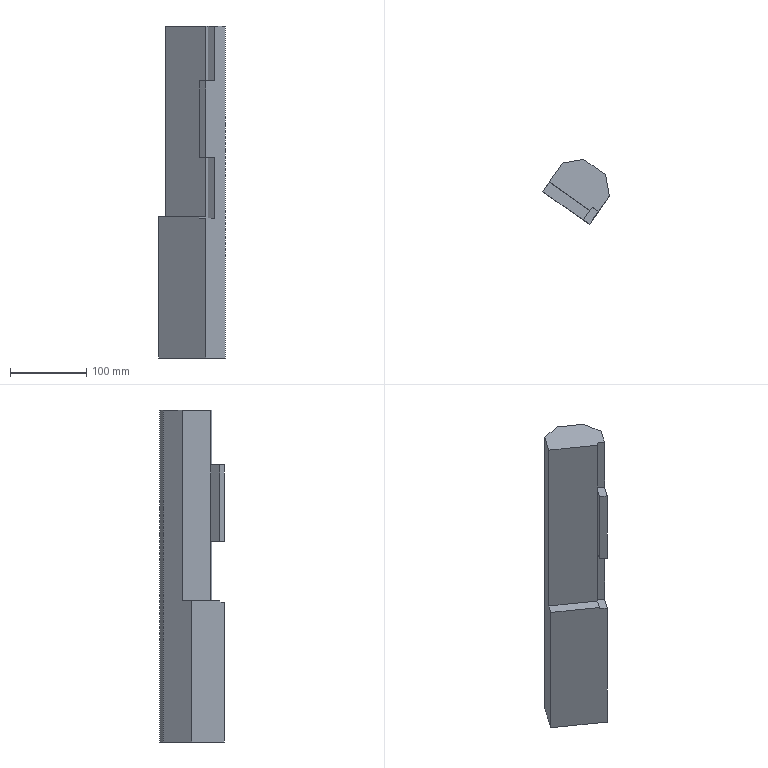Part | NX | features solid 2 | 1 solid | 19 faces | box 87.247 x 84.792 x 435 mm | volume 1672471 mm3 | plane 19
STEP:
#1=CARTESIAN_POINT('',(329.008,618.065,-154.062));
#2=VERTEX_POINT('',#1);
#3=CARTESIAN_POINT('',(357.678,597.989,-154.062));
#4=VERTEX_POINT('',#3);
#5=CARTESIAN_POINT('',(-199.131,987.872,-154.062));
#6=DIRECTION('',(0.8192,-0.5736,0.));
#7=VECTOR('',#6,1000.);
#8=LINE('',#5,#7);
#9=EDGE_CURVE('',#2,#4,#8,.T.);
#10=ORIENTED_EDGE('',*,*,#9,.F.);
#11=CARTESIAN_POINT('',(301.153,613.153,-154.062));
#12=VERTEX_POINT('',#11);
#13=CARTESIAN_POINT('',(301.153,613.153,-154.062));
#14=DIRECTION('',(-0.9848,-0.1736,0.));
#15=VECTOR('',#14,1000.);
#16=LINE('',#13,#15);
#17=EDGE_CURVE('',#2,#12,#16,.T.);
#18=ORIENTED_EDGE('',*,*,#17,.T.);
#19=CARTESIAN_POINT('',(283.946,588.579,-154.062));
#20=VERTEX_POINT('',#19);
#21=CARTESIAN_POINT('',(283.946,588.579,-154.062));
#22=DIRECTION('',(0.5736,0.8192,0.));
#23=VECTOR('',#22,1000.);
#24=LINE('',#21,#23);
#25=EDGE_CURVE('',#20,#12,#24,.T.);
#26=ORIENTED_EDGE('',*,*,#25,.F.);
#27=CARTESIAN_POINT('',(337.191,551.296,-154.062));
#28=VERTEX_POINT('',#27);
#29=CARTESIAN_POINT('',(283.946,588.579,-154.062));
#30=DIRECTION('',(0.8192,-0.5736,0.));
#31=VECTOR('',#30,1000.);
#32=LINE('',#29,#31);
#33=EDGE_CURVE('',#20,#28,#32,.T.);
#34=ORIENTED_EDGE('',*,*,#33,.T.);
#35=CARTESIAN_POINT('',(340.059,555.392,-154.062));
#36=VERTEX_POINT('',#35);
#37=CARTESIAN_POINT('',(337.191,551.296,-154.062));
#38=DIRECTION('',(-0.5736,-0.8192,0.));
#39=VECTOR('',#38,1000.);
#40=LINE('',#37,#39);
#41=EDGE_CURVE('',#36,#28,#40,.T.);
#42=ORIENTED_EDGE('',*,*,#41,.F.);
#43=CARTESIAN_POINT('',(348.25,549.656,-154.062));
#44=VERTEX_POINT('',#43);
#45=CARTESIAN_POINT('',(286.814,592.674,-154.062));
#46=DIRECTION('',(0.8192,-0.5736,0.));
#47=VECTOR('',#46,1000.);
#48=LINE('',#45,#47);
#49=EDGE_CURVE('',#36,#44,#48,.T.);
#50=ORIENTED_EDGE('',*,*,#49,.T.);
#51=CARTESIAN_POINT('',(362.59,570.135,-154.062));
#52=VERTEX_POINT('',#51);
#53=CARTESIAN_POINT('',(345.382,545.56,-154.062));
#54=DIRECTION('',(-0.5736,-0.8192,0.));
#55=VECTOR('',#54,1000.);
#56=LINE('',#53,#55);
#57=EDGE_CURVE('',#44,#52,#56,.F.);
#58=ORIENTED_EDGE('',*,*,#57,.T.);
#59=CARTESIAN_POINT('',(357.678,597.989,-154.062));
#60=DIRECTION('',(-0.1736,0.9848,0.));
#61=VECTOR('',#60,1000.);
#62=LINE('',#59,#61);
#63=EDGE_CURVE('',#52,#4,#62,.T.);
#64=ORIENTED_EDGE('',*,*,#63,.T.);
#65=EDGE_LOOP('',(#10,#18,#26,#34,#42,#50,#58,#64));
#66=FACE_BOUND('',#65,.T.);
#67=CARTESIAN_POINT('',(283.946,588.579,-154.062));
#68=DIRECTION('',(0.,0.,-1.));
#69=DIRECTION('',(0.5736,0.8192,0.));
#70=AXIS2_PLACEMENT_3D('',#67,#68,#69);
#71=PLANE('',#70);
#72=ADVANCED_FACE('',(#66),#71,.F.);
#73=CARTESIAN_POINT('',(337.191,551.296,-226.082));
#74=VERTEX_POINT('',#73);
#75=CARTESIAN_POINT('',(337.191,551.296,-326.082));
#76=VERTEX_POINT('',#75);
#77=CARTESIAN_POINT('',(337.191,551.296,-401.082));
#78=DIRECTION('',(0.,0.,-1.));
#79=VECTOR('',#78,1000.);
#80=LINE('',#77,#79);
#81=EDGE_CURVE('',#74,#76,#80,.T.);
#82=ORIENTED_EDGE('',*,*,#81,.F.);
#83=CARTESIAN_POINT('',(337.191,551.296,-401.082));
#84=DIRECTION('',(0.,0.,1.));
#85=VECTOR('',#84,1000.);
#86=LINE('',#83,#85);
#87=EDGE_CURVE('',#74,#28,#86,.T.);
#88=ORIENTED_EDGE('',*,*,#87,.T.);
#89=ORIENTED_EDGE('',*,*,#33,.F.);
#90=CARTESIAN_POINT('',(283.946,588.579,-404.062));
#91=VERTEX_POINT('',#90);
#92=CARTESIAN_POINT('',(283.946,588.579,-401.082));
#93=DIRECTION('',(0.,0.,-1.));
#94=VECTOR('',#93,1000.);
#95=LINE('',#92,#94);
#96=EDGE_CURVE('',#20,#91,#95,.T.);
#97=ORIENTED_EDGE('',*,*,#96,.T.);
#98=CARTESIAN_POINT('',(337.191,551.296,-404.062));
#99=VERTEX_POINT('',#98);
#100=CARTESIAN_POINT('',(283.946,588.579,-404.062));
#101=DIRECTION('',(-0.8192,0.5736,0.));
#102=VECTOR('',#101,1000.);
#103=LINE('',#100,#102);
#104=EDGE_CURVE('',#99,#91,#103,.T.);
#105=ORIENTED_EDGE('',*,*,#104,.F.);
#106=CARTESIAN_POINT('',(337.191,551.296,-401.082));
#107=DIRECTION('',(0.,0.,-1.));
#108=VECTOR('',#107,1000.);
#109=LINE('',#106,#108);
#110=EDGE_CURVE('',#76,#99,#109,.T.);
#111=ORIENTED_EDGE('',*,*,#110,.F.);
#112=EDGE_LOOP('',(#82,#88,#89,#97,#105,#111));
#113=FACE_BOUND('',#112,.T.);
#114=CARTESIAN_POINT('',(283.946,588.579,-401.082));
#115=DIRECTION('',(0.5736,0.8192,0.));
#116=DIRECTION('',(0.8192,-0.5736,0.));
#117=AXIS2_PLACEMENT_3D('',#114,#115,#116);
#118=PLANE('',#117);
#119=ADVANCED_FACE('',(#113),#118,.F.);
#120=CARTESIAN_POINT('',(328.587,539.009,-404.062));
#121=VERTEX_POINT('',#120);
#122=CARTESIAN_POINT('',(328.587,539.009,-406.082));
#123=VERTEX_POINT('',#122);
#124=CARTESIAN_POINT('',(328.587,539.009,-326.082));
#125=DIRECTION('',(0.,0.,-1.));
#126=VECTOR('',#125,1000.);
#127=LINE('',#124,#126);
#128=EDGE_CURVE('',#121,#123,#127,.T.);
#129=ORIENTED_EDGE('',*,*,#128,.F.);
#130=CARTESIAN_POINT('',(275.342,576.291,-404.062));
#131=VERTEX_POINT('',#130);
#132=CARTESIAN_POINT('',(328.587,539.009,-404.062));
#133=DIRECTION('',(-0.8192,0.5736,0.));
#134=VECTOR('',#133,1000.);
#135=LINE('',#132,#134);
#136=EDGE_CURVE('',#121,#131,#135,.T.);
#137=ORIENTED_EDGE('',*,*,#136,.T.);
#138=CARTESIAN_POINT('',(275.342,576.291,-589.062));
#139=VERTEX_POINT('',#138);
#140=CARTESIAN_POINT('',(275.342,576.291,-401.082));
#141=DIRECTION('',(0.,0.,-1.));
#142=VECTOR('',#141,1000.);
#143=LINE('',#140,#142);
#144=EDGE_CURVE('',#131,#139,#143,.T.);
#145=ORIENTED_EDGE('',*,*,#144,.T.);
#146=CARTESIAN_POINT('',(336.779,533.273,-589.062));
#147=VERTEX_POINT('',#146);
#148=CARTESIAN_POINT('',(275.26,576.349,-589.062));
#149=DIRECTION('',(0.8192,-0.5736,0.));
#150=VECTOR('',#149,1000.);
#151=LINE('',#148,#150);
#152=EDGE_CURVE('',#147,#139,#151,.F.);
#153=ORIENTED_EDGE('',*,*,#152,.F.);
#154=CARTESIAN_POINT('',(336.779,533.273,-406.082));
#155=VERTEX_POINT('',#154);
#156=CARTESIAN_POINT('',(336.779,533.273,-461.082));
#157=DIRECTION('',(0.,0.,1.));
#158=VECTOR('',#157,1000.);
#159=LINE('',#156,#158);
#160=EDGE_CURVE('',#155,#147,#159,.F.);
#161=ORIENTED_EDGE('',*,*,#160,.F.);
#162=CARTESIAN_POINT('',(328.587,539.009,-406.082));
#163=DIRECTION('',(0.8192,-0.5736,0.));
#164=VECTOR('',#163,1000.);
#165=LINE('',#162,#164);
#166=EDGE_CURVE('',#123,#155,#165,.T.);
#167=ORIENTED_EDGE('',*,*,#166,.F.);
#168=EDGE_LOOP('',(#129,#137,#145,#153,#161,#167));
#169=FACE_BOUND('',#168,.T.);
#170=CARTESIAN_POINT('',(328.587,539.009,-461.082));
#171=DIRECTION('',(-0.5736,-0.8192,0.));
#172=DIRECTION('',(-0.8192,0.5736,0.));
#173=AXIS2_PLACEMENT_3D('',#170,#171,#172);
#174=PLANE('',#173);
#175=ADVANCED_FACE('',(#169),#174,.T.);
#176=CARTESIAN_POINT('',(301.153,613.153,-589.062));
#177=VERTEX_POINT('',#176);
#178=CARTESIAN_POINT('',(344.171,674.59,-589.062));
#179=DIRECTION('',(-0.5736,-0.8192,0.));
#180=VECTOR('',#179,1000.);
#181=LINE('',#178,#180);
#182=EDGE_CURVE('',#139,#177,#181,.F.);
#183=ORIENTED_EDGE('',*,*,#182,.T.);
#184=CARTESIAN_POINT('',(329.008,618.065,-589.062));
#185=VERTEX_POINT('',#184);
#186=CARTESIAN_POINT('',(301.153,613.153,-589.062));
#187=DIRECTION('',(-0.9848,-0.1736,0.));
#188=VECTOR('',#187,1000.);
#189=LINE('',#186,#188);
#190=EDGE_CURVE('',#177,#185,#189,.F.);
#191=ORIENTED_EDGE('',*,*,#190,.T.);
#192=CARTESIAN_POINT('',(357.678,597.989,-589.062));
#193=VERTEX_POINT('',#192);
#194=CARTESIAN_POINT('',(-199.131,987.872,-589.062));
#195=DIRECTION('',(0.8192,-0.5736,0.));
#196=VECTOR('',#195,1000.);
#197=LINE('',#194,#196);
#198=EDGE_CURVE('',#193,#185,#197,.F.);
#199=ORIENTED_EDGE('',*,*,#198,.F.);
#200=CARTESIAN_POINT('',(362.59,570.135,-589.062));
#201=VERTEX_POINT('',#200);
#202=CARTESIAN_POINT('',(357.678,597.989,-589.062));
#203=DIRECTION('',(-0.1736,0.9848,0.));
#204=VECTOR('',#203,1000.);
#205=LINE('',#202,#204);
#206=EDGE_CURVE('',#193,#201,#205,.F.);
#207=ORIENTED_EDGE('',*,*,#206,.T.);
#208=CARTESIAN_POINT('',(256.478,418.592,-589.062));
#209=DIRECTION('',(0.5736,0.8192,0.));
#210=VECTOR('',#209,1000.);
#211=LINE('',#208,#210);
#212=EDGE_CURVE('',#147,#201,#211,.T.);
#213=ORIENTED_EDGE('',*,*,#212,.F.);
#214=ORIENTED_EDGE('',*,*,#152,.T.);
#215=EDGE_LOOP('',(#183,#191,#199,#207,#213,#214));
#216=FACE_BOUND('',#215,.T.);
#217=CARTESIAN_POINT('',(344.089,674.647,-589.062));
#218=DIRECTION('',(0.,0.,-1.));
#219=DIRECTION('',(-0.5736,-0.8192,0.));
#220=AXIS2_PLACEMENT_3D('',#217,#218,#219);
#221=PLANE('',#220);
#222=ADVANCED_FACE('',(#216),#221,.T.);
#223=ORIENTED_EDGE('',*,*,#25,.T.);
#224=CARTESIAN_POINT('',(301.153,613.153,-589.062));
#225=DIRECTION('',(0.,0.,-1.));
#226=VECTOR('',#225,1000.);
#227=LINE('',#224,#226);
#228=EDGE_CURVE('',#12,#177,#227,.T.);
#229=ORIENTED_EDGE('',*,*,#228,.T.);
#230=ORIENTED_EDGE('',*,*,#182,.F.);
#231=ORIENTED_EDGE('',*,*,#144,.F.);
#232=CARTESIAN_POINT('',(283.946,588.579,-404.062));
#233=DIRECTION('',(0.5736,0.8192,0.));
#234=VECTOR('',#233,1000.);
#235=LINE('',#232,#234);
#236=EDGE_CURVE('',#131,#91,#235,.T.);
#237=ORIENTED_EDGE('',*,*,#236,.T.);
#238=ORIENTED_EDGE('',*,*,#96,.F.);
#239=EDGE_LOOP('',(#223,#229,#230,#231,#237,#238));
#240=FACE_BOUND('',#239,.T.);
#241=CARTESIAN_POINT('',(283.946,588.579,-151.082));
#242=DIRECTION('',(-0.8192,0.5736,0.));
#243=DIRECTION('',(0.5736,0.8192,0.));
#244=AXIS2_PLACEMENT_3D('',#241,#242,#243);
#245=PLANE('',#244);
#246=ADVANCED_FACE('',(#240),#245,.T.);
#247=ORIENTED_EDGE('',*,*,#198,.T.);
#248=CARTESIAN_POINT('',(329.008,618.065,-154.062));
#249=DIRECTION('',(0.,0.,1.));
#250=VECTOR('',#249,1000.);
#251=LINE('',#248,#250);
#252=EDGE_CURVE('',#185,#2,#251,.T.);
#253=ORIENTED_EDGE('',*,*,#252,.T.);
#254=ORIENTED_EDGE('',*,*,#9,.T.);
#255=CARTESIAN_POINT('',(357.678,597.989,-192.696));
#256=DIRECTION('',(0.,0.,-1.));
#257=VECTOR('',#256,1000.);
#258=LINE('',#255,#257);
#259=EDGE_CURVE('',#4,#193,#258,.T.);
#260=ORIENTED_EDGE('',*,*,#259,.T.);
#261=EDGE_LOOP('',(#247,#253,#254,#260));
#262=FACE_BOUND('',#261,.T.);
#263=CARTESIAN_POINT('',(-199.131,987.872,-192.696));
#264=DIRECTION('',(-0.5736,-0.8192,0.));
#265=DIRECTION('',(-0.8192,0.5736,0.));
#266=AXIS2_PLACEMENT_3D('',#263,#264,#265);
#267=PLANE('',#266);
#268=ADVANCED_FACE('',(#262),#267,.F.);
#269=CARTESIAN_POINT('',(337.191,551.296,-404.062));
#270=DIRECTION('',(0.5736,0.8192,0.));
#271=VECTOR('',#270,1000.);
#272=LINE('',#269,#271);
#273=EDGE_CURVE('',#121,#99,#272,.T.);
#274=ORIENTED_EDGE('',*,*,#273,.T.);
#275=ORIENTED_EDGE('',*,*,#104,.T.);
#276=ORIENTED_EDGE('',*,*,#236,.F.);
#277=ORIENTED_EDGE('',*,*,#136,.F.);
#278=EDGE_LOOP('',(#274,#275,#276,#277));
#279=FACE_BOUND('',#278,.T.);
#280=CARTESIAN_POINT('',(337.191,551.296,-404.062));
#281=DIRECTION('',(0.,0.,1.));
#282=DIRECTION('',(-0.5736,-0.8192,0.));
#283=AXIS2_PLACEMENT_3D('',#280,#281,#282);
#284=PLANE('',#283);
#285=ADVANCED_FACE('',(#279),#284,.T.);
#286=CARTESIAN_POINT('',(348.25,549.656,-326.082));
#287=VERTEX_POINT('',#286);
#288=CARTESIAN_POINT('',(336.779,533.273,-326.082));
#289=VERTEX_POINT('',#288);
#290=CARTESIAN_POINT('',(256.478,418.592,-326.082));
#291=DIRECTION('',(0.5736,0.8192,0.));
#292=VECTOR('',#291,1000.);
#293=LINE('',#290,#292);
#294=EDGE_CURVE('',#287,#289,#293,.F.);
#295=ORIENTED_EDGE('',*,*,#294,.T.);
#296=CARTESIAN_POINT('',(328.587,539.009,-326.082));
#297=VERTEX_POINT('',#296);
#298=CARTESIAN_POINT('',(328.587,539.009,-326.082));
#299=DIRECTION('',(-0.8192,0.5736,0.));
#300=VECTOR('',#299,1000.);
#301=LINE('',#298,#300);
#302=EDGE_CURVE('',#297,#289,#301,.F.);
#303=ORIENTED_EDGE('',*,*,#302,.F.);
#304=CARTESIAN_POINT('',(337.191,551.296,-326.082));
#305=DIRECTION('',(-0.5736,-0.8192,0.));
#306=VECTOR('',#305,1000.);
#307=LINE('',#304,#306);
#308=EDGE_CURVE('',#76,#297,#307,.T.);
#309=ORIENTED_EDGE('',*,*,#308,.F.);
#310=CARTESIAN_POINT('',(340.059,555.392,-326.082));
#311=VERTEX_POINT('',#310);
#312=CARTESIAN_POINT('',(337.191,551.296,-326.082));
#313=DIRECTION('',(-0.5736,-0.8192,0.));
#314=VECTOR('',#313,1000.);
#315=LINE('',#312,#314);
#316=EDGE_CURVE('',#311,#76,#315,.T.);
#317=ORIENTED_EDGE('',*,*,#316,.F.);
#318=CARTESIAN_POINT('',(340.059,555.392,-326.082));
#319=DIRECTION('',(0.8192,-0.5736,0.));
#320=VECTOR('',#319,1000.);
#321=LINE('',#318,#320);
#322=EDGE_CURVE('',#311,#287,#321,.T.);
#323=ORIENTED_EDGE('',*,*,#322,.T.);
#324=EDGE_LOOP('',(#295,#303,#309,#317,#323));
#325=FACE_BOUND('',#324,.T.);
#326=CARTESIAN_POINT('',(337.191,551.296,-326.082));
#327=DIRECTION('',(0.,0.,-1.));
#328=DIRECTION('',(0.08716,0.9962,0.));
#329=AXIS2_PLACEMENT_3D('',#326,#327,#328);
#330=PLANE('',#329);
#331=ADVANCED_FACE('',(#325),#330,.T.);
#332=CARTESIAN_POINT('',(340.059,555.392,-226.082));
#333=VERTEX_POINT('',#332);
#334=CARTESIAN_POINT('',(348.25,549.656,-226.082));
#335=VERTEX_POINT('',#334);
#336=CARTESIAN_POINT('',(286.814,592.674,-226.082));
#337=DIRECTION('',(0.8192,-0.5736,0.));
#338=VECTOR('',#337,1000.);
#339=LINE('',#336,#338);
#340=EDGE_CURVE('',#333,#335,#339,.T.);
#341=ORIENTED_EDGE('',*,*,#340,.F.);
#342=CARTESIAN_POINT('',(337.191,551.296,-226.082));
#343=DIRECTION('',(-0.5736,-0.8192,0.));
#344=VECTOR('',#343,1000.);
#345=LINE('',#342,#344);
#346=EDGE_CURVE('',#333,#74,#345,.T.);
#347=ORIENTED_EDGE('',*,*,#346,.T.);
#348=CARTESIAN_POINT('',(328.587,539.009,-226.082));
#349=VERTEX_POINT('',#348);
#350=CARTESIAN_POINT('',(337.191,551.296,-226.082));
#351=DIRECTION('',(-0.5736,-0.8192,0.));
#352=VECTOR('',#351,1000.);
#353=LINE('',#350,#352);
#354=EDGE_CURVE('',#74,#349,#353,.T.);
#355=ORIENTED_EDGE('',*,*,#354,.T.);
#356=CARTESIAN_POINT('',(336.779,533.273,-226.082));
#357=VERTEX_POINT('',#356);
#358=CARTESIAN_POINT('',(328.587,539.009,-226.082));
#359=DIRECTION('',(-0.8192,0.5736,0.));
#360=VECTOR('',#359,1000.);
#361=LINE('',#358,#360);
#362=EDGE_CURVE('',#349,#357,#361,.F.);
#363=ORIENTED_EDGE('',*,*,#362,.T.);
#364=CARTESIAN_POINT('',(256.478,418.592,-226.082));
#365=DIRECTION('',(0.5736,0.8192,0.));
#366=VECTOR('',#365,1000.);
#367=LINE('',#364,#366);
#368=EDGE_CURVE('',#335,#357,#367,.F.);
#369=ORIENTED_EDGE('',*,*,#368,.F.);
#370=EDGE_LOOP('',(#341,#347,#355,#363,#369));
#371=FACE_BOUND('',#370,.T.);
#372=CARTESIAN_POINT('',(337.191,551.296,-226.082));
#373=DIRECTION('',(0.,0.,-1.));
#374=DIRECTION('',(0.08716,0.9962,0.));
#375=AXIS2_PLACEMENT_3D('',#372,#373,#374);
#376=PLANE('',#375);
#377=ADVANCED_FACE('',(#371),#376,.F.);
#378=ORIENTED_EDGE('',*,*,#81,.T.);
#379=ORIENTED_EDGE('',*,*,#308,.T.);
#380=CARTESIAN_POINT('',(328.587,539.009,-461.082));
#381=DIRECTION('',(0.,0.,1.));
#382=VECTOR('',#381,1000.);
#383=LINE('',#380,#382);
#384=EDGE_CURVE('',#349,#297,#383,.F.);
#385=ORIENTED_EDGE('',*,*,#384,.F.);
#386=ORIENTED_EDGE('',*,*,#354,.F.);
#387=EDGE_LOOP('',(#378,#379,#385,#386));
#388=FACE_BOUND('',#387,.T.);
#389=CARTESIAN_POINT('',(337.191,551.296,-151.082));
#390=DIRECTION('',(-0.8192,0.5736,0.));
#391=DIRECTION('',(0.5736,0.8192,0.));
#392=AXIS2_PLACEMENT_3D('',#389,#390,#391);
#393=PLANE('',#392);
#394=ADVANCED_FACE('',(#388),#393,.T.);
#395=CARTESIAN_POINT('',(336.779,533.273,-400.));
#396=DIRECTION('',(0.,0.,-1.));
#397=VECTOR('',#396,1000.);
#398=LINE('',#395,#397);
#399=EDGE_CURVE('',#357,#289,#398,.T.);
#400=ORIENTED_EDGE('',*,*,#399,.F.);
#401=ORIENTED_EDGE('',*,*,#362,.F.);
#402=ORIENTED_EDGE('',*,*,#384,.T.);
#403=ORIENTED_EDGE('',*,*,#302,.T.);
#404=EDGE_LOOP('',(#400,#401,#402,#403));
#405=FACE_BOUND('',#404,.T.);
#406=CARTESIAN_POINT('',(328.587,539.009,-461.082));
#407=DIRECTION('',(-0.5736,-0.8192,0.));
#408=DIRECTION('',(-0.8192,0.5736,0.));
#409=AXIS2_PLACEMENT_3D('',#406,#407,#408);
#410=PLANE('',#409);
#411=ADVANCED_FACE('',(#405),#410,.T.);
#412=ORIENTED_EDGE('',*,*,#212,.T.);
#413=CARTESIAN_POINT('',(362.59,570.135,-400.));
#414=DIRECTION('',(0.,0.,-1.));
#415=VECTOR('',#414,1000.);
#416=LINE('',#413,#415);
#417=EDGE_CURVE('',#201,#52,#416,.F.);
#418=ORIENTED_EDGE('',*,*,#417,.T.);
#419=ORIENTED_EDGE('',*,*,#57,.F.);
#420=CARTESIAN_POINT('',(348.25,549.656,-226.082));
#421=DIRECTION('',(0.,0.,-1.));
#422=VECTOR('',#421,1000.);
#423=LINE('',#420,#422);
#424=EDGE_CURVE('',#335,#44,#423,.F.);
#425=ORIENTED_EDGE('',*,*,#424,.F.);
#426=ORIENTED_EDGE('',*,*,#368,.T.);
#427=ORIENTED_EDGE('',*,*,#399,.T.);
#428=ORIENTED_EDGE('',*,*,#294,.F.);
#429=CARTESIAN_POINT('',(348.25,549.656,-406.082));
#430=VERTEX_POINT('',#429);
#431=CARTESIAN_POINT('',(348.25,549.656,-326.082));
#432=DIRECTION('',(0.,0.,1.));
#433=VECTOR('',#432,1000.);
#434=LINE('',#431,#433);
#435=EDGE_CURVE('',#287,#430,#434,.F.);
#436=ORIENTED_EDGE('',*,*,#435,.T.);
#437=CARTESIAN_POINT('',(345.382,545.56,-406.082));
#438=DIRECTION('',(-0.5736,-0.8192,0.));
#439=VECTOR('',#438,1000.);
#440=LINE('',#437,#439);
#441=EDGE_CURVE('',#155,#430,#440,.F.);
#442=ORIENTED_EDGE('',*,*,#441,.F.);
#443=ORIENTED_EDGE('',*,*,#160,.T.);
#444=EDGE_LOOP('',(#412,#418,#419,#425,#426,#427,#428,#436,#442,#443));
#445=FACE_BOUND('',#444,.T.);
#446=CARTESIAN_POINT('',(256.478,418.592,-400.));
#447=DIRECTION('',(0.8192,-0.5736,0.));
#448=DIRECTION('',(0.,0.,1.));
#449=AXIS2_PLACEMENT_3D('',#446,#447,#448);
#450=PLANE('',#449);
#451=ADVANCED_FACE('',(#445),#450,.T.);
#452=ORIENTED_EDGE('',*,*,#87,.F.);
#453=ORIENTED_EDGE('',*,*,#346,.F.);
#454=CARTESIAN_POINT('',(340.059,555.392,-226.082));
#455=DIRECTION('',(0.,0.,1.));
#456=VECTOR('',#455,1000.);
#457=LINE('',#454,#456);
#458=EDGE_CURVE('',#333,#36,#457,.T.);
#459=ORIENTED_EDGE('',*,*,#458,.T.);
#460=ORIENTED_EDGE('',*,*,#41,.T.);
#461=EDGE_LOOP('',(#452,#453,#459,#460));
#462=FACE_BOUND('',#461,.T.);
#463=CARTESIAN_POINT('',(337.191,551.296,-226.082));
#464=DIRECTION('',(0.8192,-0.5736,0.));
#465=DIRECTION('',(-0.5736,-0.8192,0.));
#466=AXIS2_PLACEMENT_3D('',#463,#464,#465);
#467=PLANE('',#466);
#468=ADVANCED_FACE('',(#462),#467,.T.);
#469=ORIENTED_EDGE('',*,*,#49,.F.);
#470=ORIENTED_EDGE('',*,*,#458,.F.);
#471=ORIENTED_EDGE('',*,*,#340,.T.);
#472=ORIENTED_EDGE('',*,*,#424,.T.);
#473=EDGE_LOOP('',(#469,#470,#471,#472));
#474=FACE_BOUND('',#473,.T.);
#475=CARTESIAN_POINT('',(286.814,592.674,-226.082));
#476=DIRECTION('',(0.5736,0.8192,0.));
#477=DIRECTION('',(0.8192,-0.5736,0.));
#478=AXIS2_PLACEMENT_3D('',#475,#476,#477);
#479=PLANE('',#478);
#480=ADVANCED_FACE('',(#474),#479,.F.);
#481=ORIENTED_EDGE('',*,*,#166,.T.);
#482=ORIENTED_EDGE('',*,*,#441,.T.);
#483=CARTESIAN_POINT('',(340.059,555.392,-406.082));
#484=VERTEX_POINT('',#483);
#485=CARTESIAN_POINT('',(340.059,555.392,-406.082));
#486=DIRECTION('',(0.8192,-0.5736,0.));
#487=VECTOR('',#486,1000.);
#488=LINE('',#485,#487);
#489=EDGE_CURVE('',#484,#430,#488,.T.);
#490=ORIENTED_EDGE('',*,*,#489,.F.);
#491=CARTESIAN_POINT('',(337.191,551.296,-406.082));
#492=DIRECTION('',(-0.5736,-0.8192,0.));
#493=VECTOR('',#492,1000.);
#494=LINE('',#491,#493);
#495=EDGE_CURVE('',#484,#123,#494,.T.);
#496=ORIENTED_EDGE('',*,*,#495,.T.);
#497=EDGE_LOOP('',(#481,#482,#490,#496));
#498=FACE_BOUND('',#497,.T.);
#499=CARTESIAN_POINT('',(337.191,551.296,-406.082));
#500=DIRECTION('',(0.,0.,-1.));
#501=DIRECTION('',(0.08716,0.9962,0.));
#502=AXIS2_PLACEMENT_3D('',#499,#500,#501);
#503=PLANE('',#502);
#504=ADVANCED_FACE('',(#498),#503,.F.);
#505=ORIENTED_EDGE('',*,*,#316,.T.);
#506=ORIENTED_EDGE('',*,*,#110,.T.);
#507=ORIENTED_EDGE('',*,*,#273,.F.);
#508=ORIENTED_EDGE('',*,*,#128,.T.);
#509=ORIENTED_EDGE('',*,*,#495,.F.);
#510=CARTESIAN_POINT('',(340.059,555.392,-326.082));
#511=DIRECTION('',(0.,0.,-1.));
#512=VECTOR('',#511,1000.);
#513=LINE('',#510,#512);
#514=EDGE_CURVE('',#311,#484,#513,.T.);
#515=ORIENTED_EDGE('',*,*,#514,.F.);
#516=EDGE_LOOP('',(#505,#506,#507,#508,#509,#515));
#517=FACE_BOUND('',#516,.T.);
#518=CARTESIAN_POINT('',(337.191,551.296,-326.082));
#519=DIRECTION('',(-0.8192,0.5736,0.));
#520=DIRECTION('',(0.5736,0.8192,0.));
#521=AXIS2_PLACEMENT_3D('',#518,#519,#520);
#522=PLANE('',#521);
#523=ADVANCED_FACE('',(#517),#522,.F.);
#524=ORIENTED_EDGE('',*,*,#489,.T.);
#525=ORIENTED_EDGE('',*,*,#435,.F.);
#526=ORIENTED_EDGE('',*,*,#322,.F.);
#527=ORIENTED_EDGE('',*,*,#514,.T.);
#528=EDGE_LOOP('',(#524,#525,#526,#527));
#529=FACE_BOUND('',#528,.T.);
#530=CARTESIAN_POINT('',(286.814,592.674,-326.082));
#531=DIRECTION('',(-0.5736,-0.8192,0.));
#532=DIRECTION('',(-0.8192,0.5736,0.));
#533=AXIS2_PLACEMENT_3D('',#530,#531,#532);
#534=PLANE('',#533);
#535=ADVANCED_FACE('',(#529),#534,.T.);
#536=ORIENTED_EDGE('',*,*,#63,.F.);
#537=ORIENTED_EDGE('',*,*,#417,.F.);
#538=ORIENTED_EDGE('',*,*,#206,.F.);
#539=ORIENTED_EDGE('',*,*,#259,.F.);
#540=EDGE_LOOP('',(#536,#537,#538,#539));
#541=FACE_BOUND('',#540,.T.);
#542=CARTESIAN_POINT('',(357.678,597.989,-192.696));
#543=DIRECTION('',(0.9848,0.1736,0.));
#544=DIRECTION('',(-0.1736,0.9848,0.));
#545=AXIS2_PLACEMENT_3D('',#542,#543,#544);
#546=PLANE('',#545);
#547=ADVANCED_FACE('',(#541),#546,.T.);
#548=ORIENTED_EDGE('',*,*,#17,.F.);
#549=ORIENTED_EDGE('',*,*,#252,.F.);
#550=ORIENTED_EDGE('',*,*,#190,.F.);
#551=ORIENTED_EDGE('',*,*,#228,.F.);
#552=EDGE_LOOP('',(#548,#549,#550,#551));
#553=FACE_BOUND('',#552,.T.);
#554=CARTESIAN_POINT('',(301.153,613.153,-151.082));
#555=DIRECTION('',(-0.1736,0.9848,0.));
#556=DIRECTION('',(-0.9848,-0.1736,0.));
#557=AXIS2_PLACEMENT_3D('',#554,#555,#556);
#558=PLANE('',#557);
#559=ADVANCED_FACE('',(#553),#558,.T.);
#560=CLOSED_SHELL('',(#72,#119,#175,#222,#246,#268,#285,#331,#377,#394,#411,#451,#468,#480,#504,#523,#535,#547,#559));
#561=MANIFOLD_SOLID_BREP('',#560);
#562=(LENGTH_UNIT()NAMED_UNIT(*)SI_UNIT(.MILLI.,.METRE.));
#563=UNCERTAINTY_MEASURE_WITH_UNIT(LENGTH_MEASURE(0.00001),#562,'','');
#564=(NAMED_UNIT(*)PLANE_ANGLE_UNIT()SI_UNIT($,.RADIAN.));
#565=(NAMED_UNIT(*)SI_UNIT($,.STERADIAN.)SOLID_ANGLE_UNIT());
#566=(GEOMETRIC_REPRESENTATION_CONTEXT(3)GLOBAL_UNCERTAINTY_ASSIGNED_CONTEXT((#563))GLOBAL_UNIT_ASSIGNED_CONTEXT((#562,#564,#565))REPRESENTATION_CONTEXT('',''));
#567=ADVANCED_BREP_SHAPE_REPRESENTATION('',(#561),#566);